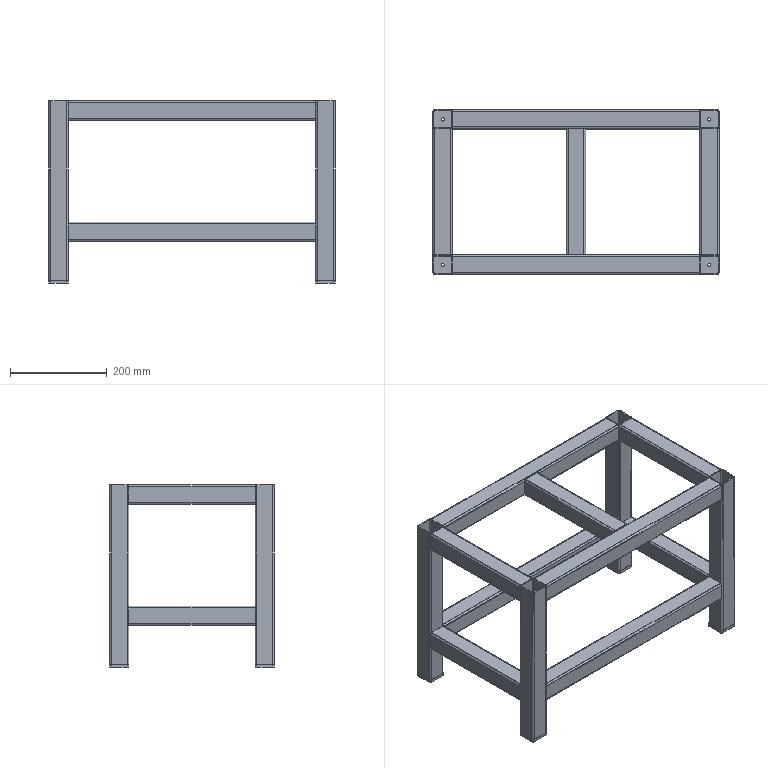Part | NX | features BREP 17 | 17 solids | 282 faces | box 590 x 340 x 376 mm | volume 1452906 mm3 | plane 154 | cylinder 128 | commonest cylinder face diameters 4 x52 8 x52 7 x16 6.8 x8